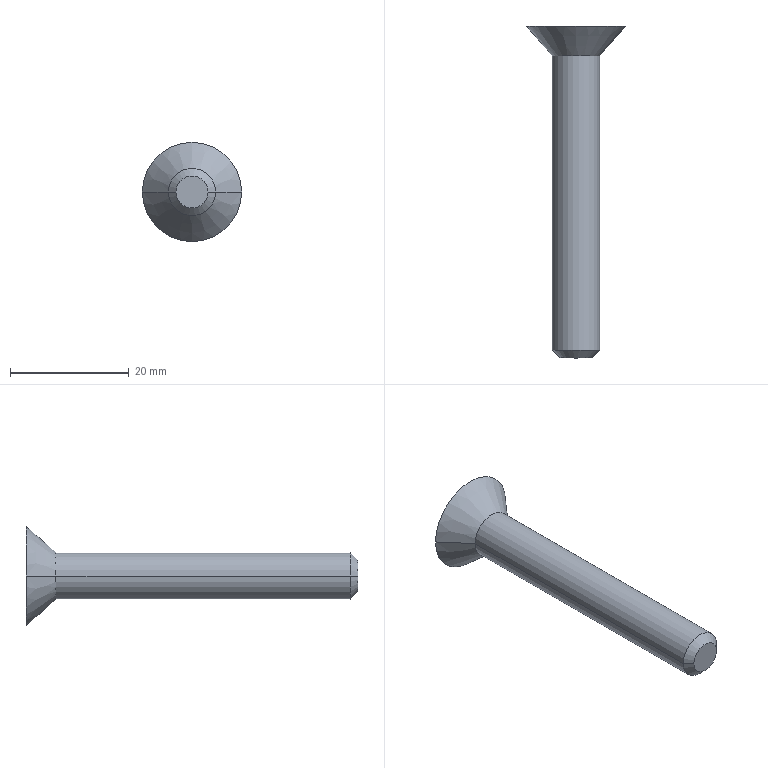Part | NX | features BREP 1 | 1 solid | 15 faces | box 16.681 x 55.829 x 16.681 mm | volume 3102 mm3 | plane 9 | cone 4 | cylinder 2 | commonest cylinder face diameters 7.938 x2
STEP:
#1=CARTESIAN_POINT('',(8.341,0.,0.));
#2=VERTEX_POINT('',#1);
#3=CARTESIAN_POINT('',(3.969,-5.029,0.));
#4=VERTEX_POINT('',#3);
#5=CARTESIAN_POINT('',(3.969,-5.029,0.));
#6=DIRECTION('',(0.6561,0.7547,0.));
#7=VECTOR('',#6,1000.);
#8=LINE('',#5,#7);
#9=EDGE_CURVE('',#2,#4,#8,.F.);
#10=ORIENTED_EDGE('',*,*,#9,.F.);
#11=CARTESIAN_POINT('',(-8.341,0.,0.));
#12=VERTEX_POINT('',#11);
#13=CARTESIAN_POINT('',(0.,0.,0.));
#14=DIRECTION('',(0.,-1.,0.));
#15=DIRECTION('',(1.,0.,0.));
#16=AXIS2_PLACEMENT_3D('',#13,#14,#15);
#17=CIRCLE('',#16,8.341);
#18=EDGE_CURVE('',#2,#12,#17,.T.);
#19=ORIENTED_EDGE('',*,*,#18,.T.);
#20=CARTESIAN_POINT('',(-3.969,-5.029,0.));
#21=VERTEX_POINT('',#20);
#22=CARTESIAN_POINT('',(-3.969,-5.029,0.));
#23=DIRECTION('',(-0.6561,0.7547,0.));
#24=VECTOR('',#23,1000.);
#25=LINE('',#22,#24);
#26=EDGE_CURVE('',#12,#21,#25,.F.);
#27=ORIENTED_EDGE('',*,*,#26,.T.);
#28=CARTESIAN_POINT('',(0.,-5.029,0.));
#29=DIRECTION('',(0.,-1.,0.));
#30=DIRECTION('',(1.,0.,0.));
#31=AXIS2_PLACEMENT_3D('',#28,#29,#30);
#32=CIRCLE('',#31,3.969);
#33=EDGE_CURVE('',#4,#21,#32,.T.);
#34=ORIENTED_EDGE('',*,*,#33,.F.);
#35=EDGE_LOOP('',(#10,#19,#27,#34));
#36=FACE_BOUND('',#35,.T.);
#37=CARTESIAN_POINT('',(0.,-2.515,0.));
#38=DIRECTION('',(0.,1.,0.));
#39=DIRECTION('',(1.,0.,0.));
#40=AXIS2_PLACEMENT_3D('',#37,#38,#39);
#41=CONICAL_SURFACE('',#40,6.155,0.7156);
#42=ADVANCED_FACE('',(#36),#41,.T.);
#43=CARTESIAN_POINT('',(-3.969,-54.559,0.));
#44=VERTEX_POINT('',#43);
#45=CARTESIAN_POINT('',(-3.969,-5.029,0.));
#46=DIRECTION('',(0.,-1.,0.));
#47=VECTOR('',#46,1000.);
#48=LINE('',#45,#47);
#49=EDGE_CURVE('',#21,#44,#48,.T.);
#50=ORIENTED_EDGE('',*,*,#49,.T.);
#51=CARTESIAN_POINT('',(3.969,-54.559,0.));
#52=VERTEX_POINT('',#51);
#53=CARTESIAN_POINT('',(0.,-54.559,0.));
#54=DIRECTION('',(0.,-1.,0.));
#55=DIRECTION('',(1.,0.,0.));
#56=AXIS2_PLACEMENT_3D('',#53,#54,#55);
#57=CIRCLE('',#56,3.969);
#58=EDGE_CURVE('',#52,#44,#57,.T.);
#59=ORIENTED_EDGE('',*,*,#58,.F.);
#60=CARTESIAN_POINT('',(3.969,-5.029,0.));
#61=DIRECTION('',(0.,-1.,0.));
#62=VECTOR('',#61,1000.);
#63=LINE('',#60,#62);
#64=EDGE_CURVE('',#4,#52,#63,.T.);
#65=ORIENTED_EDGE('',*,*,#64,.F.);
#66=ORIENTED_EDGE('',*,*,#33,.T.);
#67=EDGE_LOOP('',(#50,#59,#65,#66));
#68=FACE_BOUND('',#67,.T.);
#69=CARTESIAN_POINT('',(0.,-5.029,0.));
#70=DIRECTION('',(0.,-1.,0.));
#71=DIRECTION('',(1.,0.,0.));
#72=AXIS2_PLACEMENT_3D('',#69,#70,#71);
#73=CYLINDRICAL_SURFACE('',#72,3.969);
#74=ADVANCED_FACE('',(#68),#73,.T.);
#75=ORIENTED_EDGE('',*,*,#64,.T.);
#76=CARTESIAN_POINT('',(0.,-54.559,0.));
#77=DIRECTION('',(0.,-1.,0.));
#78=DIRECTION('',(-1.,0.,0.));
#79=AXIS2_PLACEMENT_3D('',#76,#77,#78);
#80=CIRCLE('',#79,3.969);
#81=EDGE_CURVE('',#44,#52,#80,.T.);
#82=ORIENTED_EDGE('',*,*,#81,.F.);
#83=ORIENTED_EDGE('',*,*,#49,.F.);
#84=CARTESIAN_POINT('',(0.,-5.029,0.));
#85=DIRECTION('',(0.,-1.,0.));
#86=DIRECTION('',(-1.,0.,0.));
#87=AXIS2_PLACEMENT_3D('',#84,#85,#86);
#88=CIRCLE('',#87,3.969);
#89=EDGE_CURVE('',#21,#4,#88,.T.);
#90=ORIENTED_EDGE('',*,*,#89,.T.);
#91=EDGE_LOOP('',(#75,#82,#83,#90));
#92=FACE_BOUND('',#91,.T.);
#93=CARTESIAN_POINT('',(0.,-5.029,0.));
#94=DIRECTION('',(0.,-1.,0.));
#95=DIRECTION('',(1.,0.,0.));
#96=AXIS2_PLACEMENT_3D('',#93,#94,#95);
#97=CYLINDRICAL_SURFACE('',#96,3.969);
#98=ADVANCED_FACE('',(#92),#97,.T.);
#99=ORIENTED_EDGE('',*,*,#26,.F.);
#100=CARTESIAN_POINT('',(0.,0.,0.));
#101=DIRECTION('',(0.,1.,0.));
#102=DIRECTION('',(1.,0.,0.));
#103=AXIS2_PLACEMENT_3D('',#100,#101,#102);
#104=CIRCLE('',#103,8.341);
#105=EDGE_CURVE('',#2,#12,#104,.T.);
#106=ORIENTED_EDGE('',*,*,#105,.F.);
#107=ORIENTED_EDGE('',*,*,#9,.T.);
#108=ORIENTED_EDGE('',*,*,#89,.F.);
#109=EDGE_LOOP('',(#99,#106,#107,#108));
#110=FACE_BOUND('',#109,.T.);
#111=CARTESIAN_POINT('',(0.,-2.515,0.));
#112=DIRECTION('',(0.,1.,0.));
#113=DIRECTION('',(1.,0.,0.));
#114=AXIS2_PLACEMENT_3D('',#111,#112,#113);
#115=CONICAL_SURFACE('',#114,6.155,0.7156);
#116=ADVANCED_FACE('',(#110),#115,.T.);
#117=ORIENTED_EDGE('',*,*,#18,.F.);
#118=ORIENTED_EDGE('',*,*,#105,.T.);
#119=EDGE_LOOP('',(#117,#118));
#120=FACE_BOUND('',#119,.T.);
#121=CARTESIAN_POINT('',(-1.984,0.,-1.146));
#122=VERTEX_POINT('',#121);
#123=CARTESIAN_POINT('',(-1.984,0.,1.146));
#124=VERTEX_POINT('',#123);
#125=CARTESIAN_POINT('',(-1.984,0.,-1.146));
#126=DIRECTION('',(0.,0.,1.));
#127=VECTOR('',#126,1000.);
#128=LINE('',#125,#127);
#129=EDGE_CURVE('',#122,#124,#128,.T.);
#130=ORIENTED_EDGE('',*,*,#129,.F.);
#131=CARTESIAN_POINT('',(0.,0.,-2.291));
#132=VERTEX_POINT('',#131);
#133=CARTESIAN_POINT('',(0.,0.,-2.291));
#134=DIRECTION('',(-0.866,0.,0.5));
#135=VECTOR('',#134,1000.);
#136=LINE('',#133,#135);
#137=EDGE_CURVE('',#132,#122,#136,.T.);
#138=ORIENTED_EDGE('',*,*,#137,.F.);
#139=CARTESIAN_POINT('',(1.984,0.,-1.146));
#140=VERTEX_POINT('',#139);
#141=CARTESIAN_POINT('',(1.984,0.,-1.146));
#142=DIRECTION('',(-0.866,0.,-0.5));
#143=VECTOR('',#142,1000.);
#144=LINE('',#141,#143);
#145=EDGE_CURVE('',#140,#132,#144,.T.);
#146=ORIENTED_EDGE('',*,*,#145,.F.);
#147=CARTESIAN_POINT('',(1.984,0.,1.146));
#148=VERTEX_POINT('',#147);
#149=CARTESIAN_POINT('',(1.984,0.,1.146));
#150=DIRECTION('',(0.,0.,-1.));
#151=VECTOR('',#150,1000.);
#152=LINE('',#149,#151);
#153=EDGE_CURVE('',#148,#140,#152,.T.);
#154=ORIENTED_EDGE('',*,*,#153,.F.);
#155=CARTESIAN_POINT('',(0.,0.,2.291));
#156=VERTEX_POINT('',#155);
#157=CARTESIAN_POINT('',(0.,0.,2.291));
#158=DIRECTION('',(0.866,0.,-0.5));
#159=VECTOR('',#158,1000.);
#160=LINE('',#157,#159);
#161=EDGE_CURVE('',#156,#148,#160,.T.);
#162=ORIENTED_EDGE('',*,*,#161,.F.);
#163=CARTESIAN_POINT('',(-1.984,0.,1.146));
#164=DIRECTION('',(0.866,0.,0.5));
#165=VECTOR('',#164,1000.);
#166=LINE('',#163,#165);
#167=EDGE_CURVE('',#124,#156,#166,.T.);
#168=ORIENTED_EDGE('',*,*,#167,.F.);
#169=EDGE_LOOP('',(#130,#138,#146,#154,#162,#168));
#170=FACE_BOUND('',#169,.T.);
#171=CARTESIAN_POINT('',(0.,0.,0.));
#172=DIRECTION('',(0.,-1.,0.));
#173=DIRECTION('',(0.,0.,-1.));
#174=AXIS2_PLACEMENT_3D('',#171,#172,#173);
#175=PLANE('',#174);
#176=ADVANCED_FACE('',(#120,#170),#175,.F.);
#177=CARTESIAN_POINT('',(0.,-1.27,2.291));
#178=VERTEX_POINT('',#177);
#179=CARTESIAN_POINT('',(0.,0.,2.291));
#180=DIRECTION('',(0.,-1.,0.));
#181=VECTOR('',#180,1000.);
#182=LINE('',#179,#181);
#183=EDGE_CURVE('',#156,#178,#182,.T.);
#184=ORIENTED_EDGE('',*,*,#183,.T.);
#185=CARTESIAN_POINT('',(-1.984,-1.27,1.146));
#186=VERTEX_POINT('',#185);
#187=CARTESIAN_POINT('',(-1.984,-1.27,1.146));
#188=DIRECTION('',(0.866,0.,0.5));
#189=VECTOR('',#188,1000.);
#190=LINE('',#187,#189);
#191=EDGE_CURVE('',#186,#178,#190,.T.);
#192=ORIENTED_EDGE('',*,*,#191,.F.);
#193=CARTESIAN_POINT('',(-1.984,0.,1.146));
#194=DIRECTION('',(0.,-1.,0.));
#195=VECTOR('',#194,1000.);
#196=LINE('',#193,#195);
#197=EDGE_CURVE('',#124,#186,#196,.T.);
#198=ORIENTED_EDGE('',*,*,#197,.F.);
#199=ORIENTED_EDGE('',*,*,#167,.T.);
#200=EDGE_LOOP('',(#184,#192,#198,#199));
#201=FACE_BOUND('',#200,.T.);
#202=CARTESIAN_POINT('',(-1.984,0.,1.146));
#203=DIRECTION('',(-0.5,0.,0.866));
#204=DIRECTION('',(0.,1.,0.));
#205=AXIS2_PLACEMENT_3D('',#202,#203,#204);
#206=PLANE('',#205);
#207=ADVANCED_FACE('',(#201),#206,.F.);
#208=ORIENTED_EDGE('',*,*,#197,.T.);
#209=CARTESIAN_POINT('',(-1.984,-1.27,-1.146));
#210=VERTEX_POINT('',#209);
#211=CARTESIAN_POINT('',(-1.984,-1.27,-1.146));
#212=DIRECTION('',(0.,0.,1.));
#213=VECTOR('',#212,1000.);
#214=LINE('',#211,#213);
#215=EDGE_CURVE('',#210,#186,#214,.T.);
#216=ORIENTED_EDGE('',*,*,#215,.F.);
#217=CARTESIAN_POINT('',(-1.984,0.,-1.146));
#218=DIRECTION('',(0.,-1.,0.));
#219=VECTOR('',#218,1000.);
#220=LINE('',#217,#219);
#221=EDGE_CURVE('',#122,#210,#220,.T.);
#222=ORIENTED_EDGE('',*,*,#221,.F.);
#223=ORIENTED_EDGE('',*,*,#129,.T.);
#224=EDGE_LOOP('',(#208,#216,#222,#223));
#225=FACE_BOUND('',#224,.T.);
#226=CARTESIAN_POINT('',(-1.984,0.,-1.146));
#227=DIRECTION('',(-1.,0.,0.));
#228=DIRECTION('',(0.,0.,1.));
#229=AXIS2_PLACEMENT_3D('',#226,#227,#228);
#230=PLANE('',#229);
#231=ADVANCED_FACE('',(#225),#230,.F.);
#232=ORIENTED_EDGE('',*,*,#221,.T.);
#233=CARTESIAN_POINT('',(0.,-1.27,-2.291));
#234=VERTEX_POINT('',#233);
#235=CARTESIAN_POINT('',(0.,-1.27,-2.291));
#236=DIRECTION('',(-0.866,0.,0.5));
#237=VECTOR('',#236,1000.);
#238=LINE('',#235,#237);
#239=EDGE_CURVE('',#234,#210,#238,.T.);
#240=ORIENTED_EDGE('',*,*,#239,.F.);
#241=CARTESIAN_POINT('',(0.,0.,-2.291));
#242=DIRECTION('',(0.,-1.,0.));
#243=VECTOR('',#242,1000.);
#244=LINE('',#241,#243);
#245=EDGE_CURVE('',#132,#234,#244,.T.);
#246=ORIENTED_EDGE('',*,*,#245,.F.);
#247=ORIENTED_EDGE('',*,*,#137,.T.);
#248=EDGE_LOOP('',(#232,#240,#246,#247));
#249=FACE_BOUND('',#248,.T.);
#250=CARTESIAN_POINT('',(0.,0.,-2.291));
#251=DIRECTION('',(-0.5,0.,-0.866));
#252=DIRECTION('',(-0.866,0.,0.5));
#253=AXIS2_PLACEMENT_3D('',#250,#251,#252);
#254=PLANE('',#253);
#255=ADVANCED_FACE('',(#249),#254,.F.);
#256=ORIENTED_EDGE('',*,*,#245,.T.);
#257=CARTESIAN_POINT('',(1.984,-1.27,-1.146));
#258=VERTEX_POINT('',#257);
#259=CARTESIAN_POINT('',(1.984,-1.27,-1.146));
#260=DIRECTION('',(-0.866,0.,-0.5));
#261=VECTOR('',#260,1000.);
#262=LINE('',#259,#261);
#263=EDGE_CURVE('',#258,#234,#262,.T.);
#264=ORIENTED_EDGE('',*,*,#263,.F.);
#265=CARTESIAN_POINT('',(1.984,0.,-1.146));
#266=DIRECTION('',(0.,-1.,0.));
#267=VECTOR('',#266,1000.);
#268=LINE('',#265,#267);
#269=EDGE_CURVE('',#140,#258,#268,.T.);
#270=ORIENTED_EDGE('',*,*,#269,.F.);
#271=ORIENTED_EDGE('',*,*,#145,.T.);
#272=EDGE_LOOP('',(#256,#264,#270,#271));
#273=FACE_BOUND('',#272,.T.);
#274=CARTESIAN_POINT('',(1.984,0.,-1.146));
#275=DIRECTION('',(0.5,0.,-0.866));
#276=DIRECTION('',(0.,-1.,0.));
#277=AXIS2_PLACEMENT_3D('',#274,#275,#276);
#278=PLANE('',#277);
#279=ADVANCED_FACE('',(#273),#278,.F.);
#280=ORIENTED_EDGE('',*,*,#269,.T.);
#281=CARTESIAN_POINT('',(1.984,-1.27,1.146));
#282=VERTEX_POINT('',#281);
#283=CARTESIAN_POINT('',(1.984,-1.27,1.146));
#284=DIRECTION('',(0.,0.,-1.));
#285=VECTOR('',#284,1000.);
#286=LINE('',#283,#285);
#287=EDGE_CURVE('',#282,#258,#286,.T.);
#288=ORIENTED_EDGE('',*,*,#287,.F.);
#289=CARTESIAN_POINT('',(1.984,0.,1.146));
#290=DIRECTION('',(0.,-1.,0.));
#291=VECTOR('',#290,1000.);
#292=LINE('',#289,#291);
#293=EDGE_CURVE('',#148,#282,#292,.T.);
#294=ORIENTED_EDGE('',*,*,#293,.F.);
#295=ORIENTED_EDGE('',*,*,#153,.T.);
#296=EDGE_LOOP('',(#280,#288,#294,#295));
#297=FACE_BOUND('',#296,.T.);
#298=CARTESIAN_POINT('',(1.984,0.,1.146));
#299=DIRECTION('',(1.,0.,0.));
#300=DIRECTION('',(0.,1.,0.));
#301=AXIS2_PLACEMENT_3D('',#298,#299,#300);
#302=PLANE('',#301);
#303=ADVANCED_FACE('',(#297),#302,.F.);
#304=ORIENTED_EDGE('',*,*,#293,.T.);
#305=CARTESIAN_POINT('',(0.,-1.27,2.291));
#306=DIRECTION('',(0.866,0.,-0.5));
#307=VECTOR('',#306,1000.);
#308=LINE('',#305,#307);
#309=EDGE_CURVE('',#178,#282,#308,.T.);
#310=ORIENTED_EDGE('',*,*,#309,.F.);
#311=ORIENTED_EDGE('',*,*,#183,.F.);
#312=ORIENTED_EDGE('',*,*,#161,.T.);
#313=EDGE_LOOP('',(#304,#310,#311,#312));
#314=FACE_BOUND('',#313,.T.);
#315=CARTESIAN_POINT('',(0.,0.,2.291));
#316=DIRECTION('',(0.5,0.,0.866));
#317=DIRECTION('',(0.,-1.,0.));
#318=AXIS2_PLACEMENT_3D('',#315,#316,#317);
#319=PLANE('',#318);
#320=ADVANCED_FACE('',(#314),#319,.F.);
#321=ORIENTED_EDGE('',*,*,#309,.T.);
#322=ORIENTED_EDGE('',*,*,#287,.T.);
#323=ORIENTED_EDGE('',*,*,#263,.T.);
#324=ORIENTED_EDGE('',*,*,#239,.T.);
#325=ORIENTED_EDGE('',*,*,#215,.T.);
#326=ORIENTED_EDGE('',*,*,#191,.T.);
#327=EDGE_LOOP('',(#321,#322,#323,#324,#325,#326));
#328=FACE_BOUND('',#327,.T.);
#329=CARTESIAN_POINT('',(0.,-1.27,0.));
#330=DIRECTION('',(0.,1.,0.));
#331=DIRECTION('',(1.,0.,0.));
#332=AXIS2_PLACEMENT_3D('',#329,#330,#331);
#333=PLANE('',#332);
#334=ADVANCED_FACE('',(#328),#333,.T.);
#335=CARTESIAN_POINT('',(-2.699,-55.829,0.));
#336=VERTEX_POINT('',#335);
#337=CARTESIAN_POINT('',(-2.699,-55.829,0.));
#338=DIRECTION('',(-0.7071,0.7071,0.));
#339=VECTOR('',#338,1000.);
#340=LINE('',#337,#339);
#341=EDGE_CURVE('',#336,#44,#340,.T.);
#342=ORIENTED_EDGE('',*,*,#341,.T.);
#343=ORIENTED_EDGE('',*,*,#81,.T.);
#344=CARTESIAN_POINT('',(2.699,-55.829,0.));
#345=VERTEX_POINT('',#344);
#346=CARTESIAN_POINT('',(2.699,-55.829,0.));
#347=DIRECTION('',(0.7071,0.7071,0.));
#348=VECTOR('',#347,1000.);
#349=LINE('',#346,#348);
#350=EDGE_CURVE('',#345,#52,#349,.T.);
#351=ORIENTED_EDGE('',*,*,#350,.F.);
#352=CARTESIAN_POINT('',(0.,-55.829,0.));
#353=DIRECTION('',(0.,-1.,0.));
#354=DIRECTION('',(-1.,0.,0.));
#355=AXIS2_PLACEMENT_3D('',#352,#353,#354);
#356=CIRCLE('',#355,2.699);
#357=EDGE_CURVE('',#336,#345,#356,.T.);
#358=ORIENTED_EDGE('',*,*,#357,.F.);
#359=EDGE_LOOP('',(#342,#343,#351,#358));
#360=FACE_BOUND('',#359,.T.);
#361=CARTESIAN_POINT('',(0.,-55.194,0.));
#362=DIRECTION('',(0.,1.,0.));
#363=DIRECTION('',(-1.,0.,0.));
#364=AXIS2_PLACEMENT_3D('',#361,#362,#363);
#365=CONICAL_SURFACE('',#364,3.334,0.7854);
#366=ADVANCED_FACE('',(#360),#365,.T.);
#367=ORIENTED_EDGE('',*,*,#357,.T.);
#368=CARTESIAN_POINT('',(0.,-55.829,0.));
#369=DIRECTION('',(0.,-1.,0.));
#370=DIRECTION('',(1.,0.,0.));
#371=AXIS2_PLACEMENT_3D('',#368,#369,#370);
#372=CIRCLE('',#371,2.699);
#373=EDGE_CURVE('',#345,#336,#372,.T.);
#374=ORIENTED_EDGE('',*,*,#373,.T.);
#375=EDGE_LOOP('',(#367,#374));
#376=FACE_BOUND('',#375,.T.);
#377=CARTESIAN_POINT('',(0.,-55.829,0.));
#378=DIRECTION('',(0.,-1.,0.));
#379=DIRECTION('',(0.,0.,-1.));
#380=AXIS2_PLACEMENT_3D('',#377,#378,#379);
#381=PLANE('',#380);
#382=ADVANCED_FACE('',(#376),#381,.T.);
#383=ORIENTED_EDGE('',*,*,#350,.T.);
#384=ORIENTED_EDGE('',*,*,#58,.T.);
#385=ORIENTED_EDGE('',*,*,#341,.F.);
#386=ORIENTED_EDGE('',*,*,#373,.F.);
#387=EDGE_LOOP('',(#383,#384,#385,#386));
#388=FACE_BOUND('',#387,.T.);
#389=CARTESIAN_POINT('',(0.,-55.194,0.));
#390=DIRECTION('',(0.,1.,0.));
#391=DIRECTION('',(-1.,0.,0.));
#392=AXIS2_PLACEMENT_3D('',#389,#390,#391);
#393=CONICAL_SURFACE('',#392,3.334,0.7854);
#394=ADVANCED_FACE('',(#388),#393,.T.);
#395=CLOSED_SHELL('',(#42,#74,#98,#116,#176,#207,#231,#255,#279,#303,#320,#334,#366,#382,#394));
#396=MANIFOLD_SOLID_BREP('',#395);
#397=(LENGTH_UNIT()NAMED_UNIT(*)SI_UNIT(.MILLI.,.METRE.));
#398=UNCERTAINTY_MEASURE_WITH_UNIT(LENGTH_MEASURE(0.00001),#397,'','');
#399=(NAMED_UNIT(*)PLANE_ANGLE_UNIT()SI_UNIT($,.RADIAN.));
#400=(NAMED_UNIT(*)SI_UNIT($,.STERADIAN.)SOLID_ANGLE_UNIT());
#401=(GEOMETRIC_REPRESENTATION_CONTEXT(3)GLOBAL_UNCERTAINTY_ASSIGNED_CONTEXT((#398))GLOBAL_UNIT_ASSIGNED_CONTEXT((#397,#399,#400))REPRESENTATION_CONTEXT('',''));
#402=ADVANCED_BREP_SHAPE_REPRESENTATION('',(#396),#401);